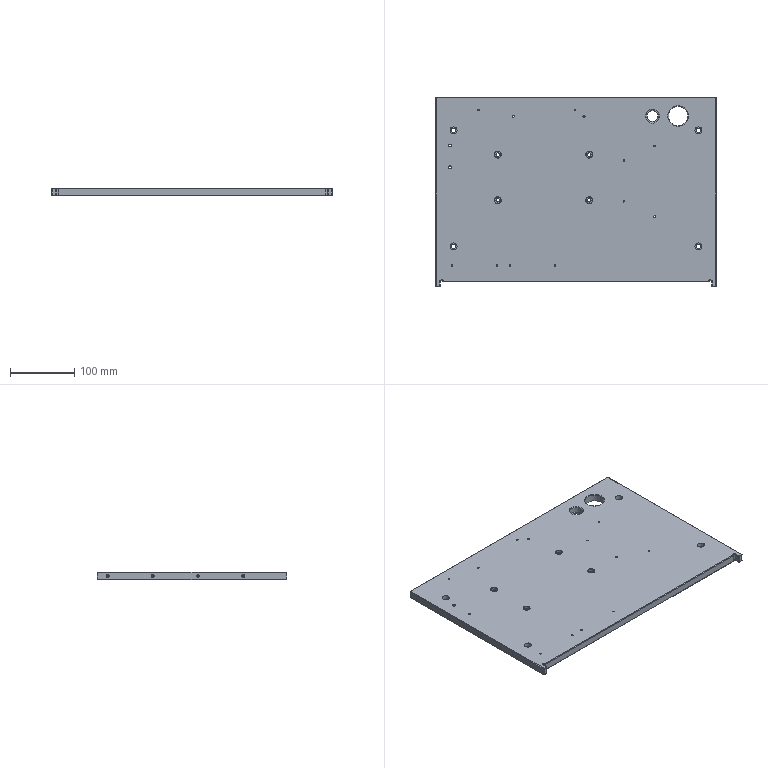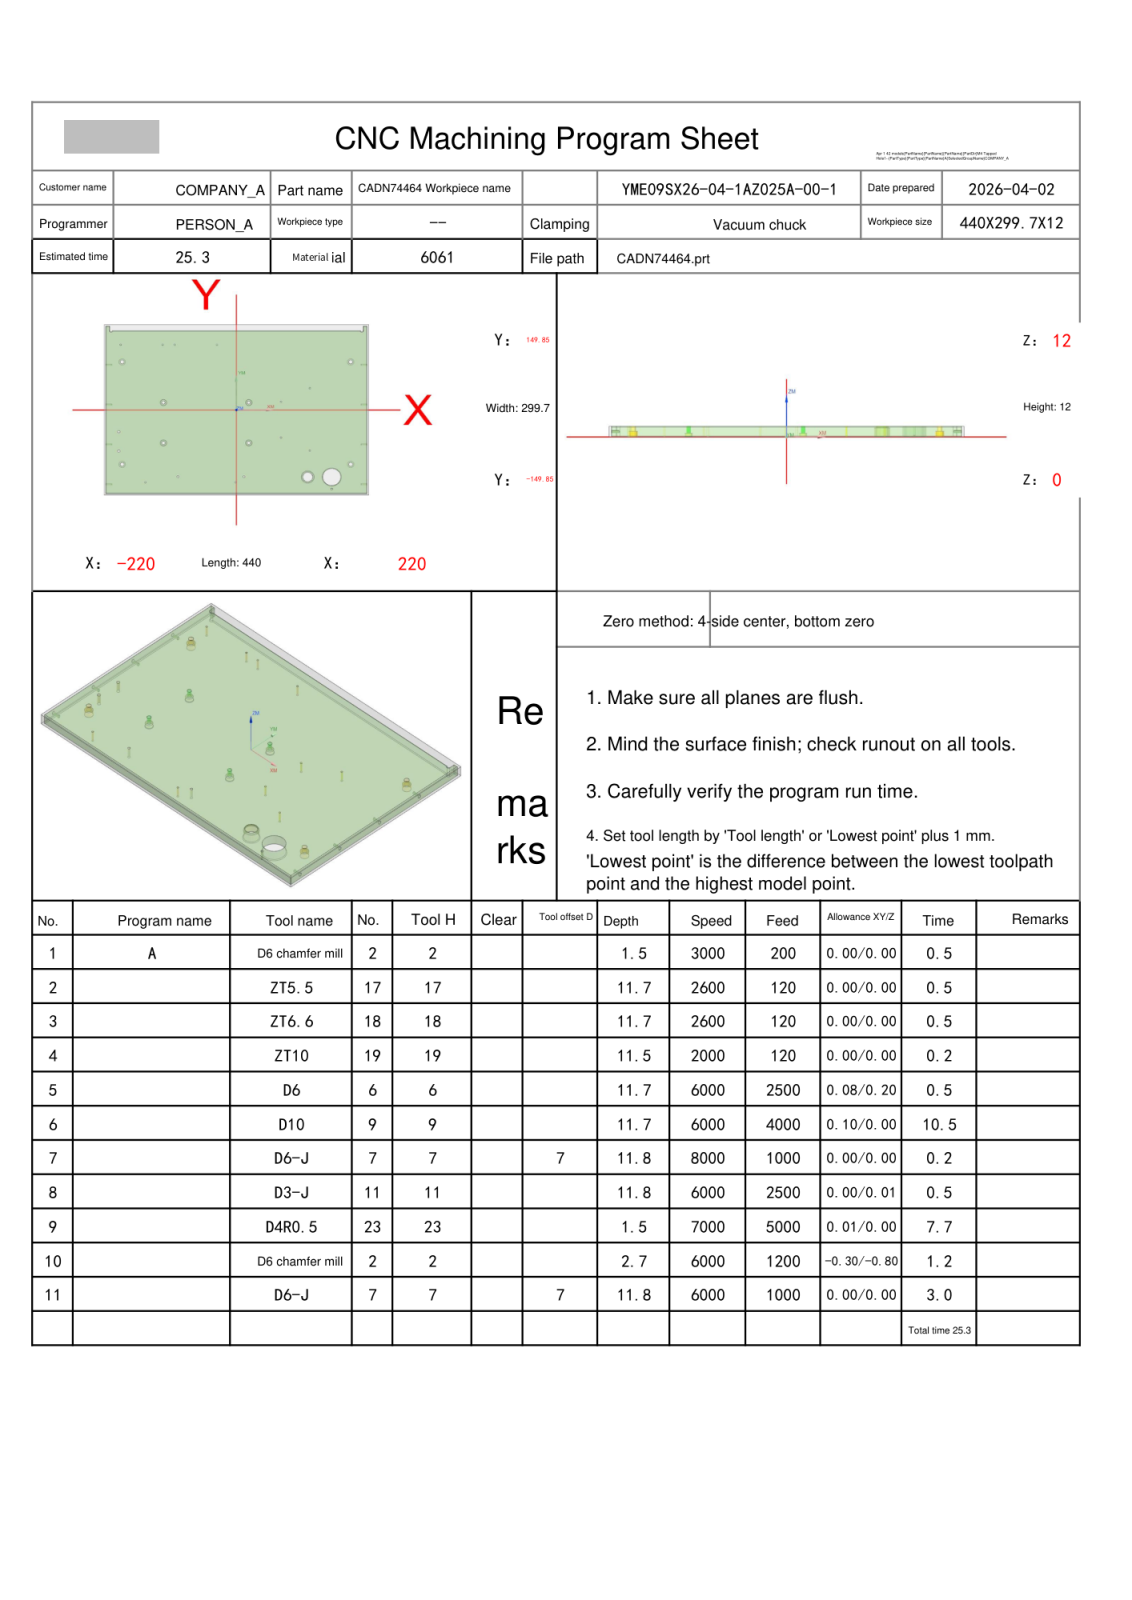NC program | NX | posted by the shop | part box 435 x 294.7 x 12 mm
Lines 896 to 1853 of 24066:
N8 T11 M06
(D3-J  D=3. R=0. H=11 ce=0.00 di=0.01)
G00 G90 G54 X-208.966 Y139.65 M03 S6000
G43 H11 Z32.
M08
Z12.471
G01 X-208.97 Y139.649 Z12.399 F2000.
X-208.981 Y139.647 Z12.326
X-208.999 Y139.642 Z12.253
X-209.022 Y139.635 Z12.182
X-209.049 Y139.626 Z12.112
X-209.078 Y139.614 Z12.046
X-209.11 Y139.599 Z11.983
X-209.142 Y139.581 Z11.924
X-209.173 Y139.559 Z11.871
X-209.203 Y139.534 Z11.824
X-209.23 Y139.506 Z11.783
X-209.253 Y139.473 Z11.75
X-209.27 Y139.437 Z11.726
X-209.282 Y139.396 Z11.71
X-209.286 Y139.35 Z11.705
G03 X-208.5 Y138.564 I.786 J0.0 F2500.
X-207.72 Y139.252 I0.0 J.786
G01 X-207.725 Y139.305 Z11.71
X-207.749 Y139.355 Z11.722
X-207.789 Y139.4 Z11.739
X-207.842 Y139.441 Z11.759
X-207.905 Y139.477 Z11.78
X-207.972 Y139.509 Z11.8
X-208.041 Y139.537 Z11.816
X-208.109 Y139.561 Z11.826
X-208.206 Y139.589 Z11.825
X-208.297 Y139.606 Z11.806
X-208.387 Y139.613 Z11.771
X-208.484 Y139.61 Z11.723
X-208.595 Y139.597 Z11.663
X-208.665 Y139.586 Z11.626
X-208.738 Y139.571 Z11.587
X-208.811 Y139.553 Z11.549
X-208.882 Y139.531 Z11.513
X-208.947 Y139.505 Z11.48
X-209.003 Y139.474 Z11.452
X-209.047 Y139.438 Z11.429
X-209.075 Y139.397 Z11.415
X-209.086 Y139.35 Z11.41
G03 X-208.5 Y138.764 I.586 J0.0
X-207.915 Y139.326 I0.0 J.586
G01 X-207.923 Y139.379 Z11.412
X-207.95 Y139.427 Z11.416
X-207.991 Y139.47 Z11.421
X-208.043 Y139.508 Z11.427
X-208.101 Y139.541 Z11.432
X-208.163 Y139.569 Z11.435
X-208.223 Y139.592
X-208.278 Y139.611 Z11.431
X-208.34 Y139.629 Z11.418
X-208.391 Y139.64 Z11.398
X-208.437 Y139.644 Z11.371
X-208.484 Y139.641 Z11.34
X-208.538 Y139.631 Z11.305
X-208.604 Y139.615 Z11.268
X-208.657 Y139.601 Z11.243
X-208.714 Y139.583 Z11.219
X-208.774 Y139.562 Z11.195
X-208.832 Y139.538 Z11.173
X-208.887 Y139.509 Z11.154
X-208.935 Y139.477 Z11.138
X-208.972 Y139.439 Z11.126
X-208.997 Y139.397 Z11.118
X-209.006 Y139.35 Z11.115
G03 X-208.5 Y138.844 I.506 J0.0
X-207.994 Y139.348 I0.0 J.506
G01 X-208.001 Y139.41 Z11.114
X-208.019 Y139.503 Z11.113
X-208.147 Y140.018 Z11.098
X-208.227 Y140.353 Z11.086
X-208.358 Y141.004 Z11.059
X-208.471 Y141.96 Z11.006
X-208.567 Y142.911 Z10.944
X-208.633 Y143.352 Z10.913
X-208.705 Y143.69 Z10.889
X-208.752 Y143.871 Z10.876
X-208.819 Y144.099 Z10.859
X-208.885 Y144.29 Z10.843
X-208.922 Y144.383 Z10.835
X-208.954 Y144.45 Z10.829
X-208.978 Y144.49 Z10.824
X-208.994 Y144.499 Z10.821
X-209. Y144.475 Z10.82
Y139.35
G03 X-208.5 Y138.85 I.5 J0.0
X-208. Y139.35 I0.0 J.5
G02 X-206.5 Y140.85 I1.5 J0.0
G01 X-205.375
X-205.346 Y140.866 Z10.819
X-205.341 Y140.911 Z10.817
X-205.358 Y140.983 Z10.812
X-205.394 Y141.078 Z10.807
X-205.449 Y141.193 Z10.8
X-205.52 Y141.325 Z10.792
X-205.702 Y141.623 Z10.774
X-205.831 Y141.816 Z10.761
X-206.055 Y142.129 Z10.74
X-206.427 Y142.585 Z10.707
X-206.833 Y143.019 Z10.673
X-207.267 Y143.425 Z10.638
X-207.722 Y143.797 Z10.605
X-208.035 Y144.021 Z10.584
X-208.228 Y144.149 Z10.571
X-208.525 Y144.331 Z10.553
X-208.657 Y144.402 Z10.545
X-208.772 Y144.456 Z10.538
X-208.867 Y144.492 Z10.533
X-208.939 Y144.509 Z10.528
X-208.984 Y144.504 Z10.526
X-209. Y144.475 Z10.525
Y139.35
G03 X-208.5 Y138.85 I.5 J0.0
X-208. Y139.35 I0.0 J.5
G02 X-206.5 Y140.85 I1.5 J0.0
G01 X-205.375
X-205.346 Y140.866 Z10.524
X-205.341 Y140.911 Z10.522
X-205.358 Y140.983 Z10.517
X-205.394 Y141.078 Z10.512
X-205.449 Y141.193 Z10.505
X-205.52 Y141.325 Z10.497
X-205.702 Y141.623 Z10.479
X-205.831 Y141.816 Z10.466
X-206.055 Y142.129 Z10.445
X-206.427 Y142.585 Z10.412
X-206.833 Y143.019 Z10.378
X-207.267 Y143.425 Z10.343
X-207.722 Y143.797 Z10.31
X-208.035 Y144.021 Z10.289
X-208.228 Y144.149 Z10.276
X-208.525 Y144.331 Z10.258
X-208.657 Y144.402 Z10.25
X-208.772 Y144.456 Z10.243
X-208.867 Y144.492 Z10.238
X-208.939 Y144.509 Z10.233
X-208.984 Y144.504 Z10.231
X-209. Y144.475 Z10.23
Y139.35
G03 X-208.5 Y138.85 I.5 J0.0
X-208. Y139.35 I0.0 J.5
G02 X-206.5 Y140.85 I1.5 J0.0
G01 X-205.375
X-205.346 Y140.866 Z10.229
X-205.341 Y140.911 Z10.227
X-205.358 Y140.983 Z10.222
X-205.394 Y141.078 Z10.217
X-205.449 Y141.193 Z10.21
X-205.52 Y141.325 Z10.202
X-205.702 Y141.623 Z10.184
X-205.831 Y141.816 Z10.171
X-206.055 Y142.129 Z10.15
X-206.427 Y142.585 Z10.117
X-206.833 Y143.019 Z10.083
X-207.267 Y143.425 Z10.048
X-207.722 Y143.797 Z10.015
X-208.035 Y144.021 Z9.994
X-208.228 Y144.149 Z9.981
X-208.525 Y144.331 Z9.963
X-208.657 Y144.402 Z9.955
X-208.772 Y144.456 Z9.948
X-208.867 Y144.492 Z9.943
X-208.939 Y144.509 Z9.938
X-208.984 Y144.504 Z9.936
X-209. Y144.475 Z9.935
Y139.35
G03 X-208.5 Y138.85 I.5 J0.0
X-208. Y139.35 I0.0 J.5
G02 X-206.5 Y140.85 I1.5 J0.0
G01 X-205.375
X-205.346 Y140.866 Z9.934
X-205.341 Y140.911 Z9.932
X-205.358 Y140.983 Z9.927
X-205.394 Y141.078 Z9.922
X-205.449 Y141.193 Z9.915
X-205.52 Y141.325 Z9.907
X-205.702 Y141.623 Z9.889
X-205.831 Y141.816 Z9.876
X-206.055 Y142.129 Z9.855
X-206.427 Y142.585 Z9.822
X-206.833 Y143.019 Z9.788
X-207.267 Y143.425 Z9.753
X-207.722 Y143.797 Z9.72
X-208.035 Y144.021 Z9.699
X-208.228 Y144.149 Z9.686
X-208.525 Y144.331 Z9.668
X-208.657 Y144.402 Z9.66
X-208.772 Y144.456 Z9.653
X-208.867 Y144.492 Z9.648
X-208.939 Y144.509 Z9.643
X-208.984 Y144.504 Z9.641
X-209. Y144.475 Z9.64
Y139.35
G03 X-208.5 Y138.85 I.5 J0.0
X-208. Y139.35 I0.0 J.5
G02 X-206.5 Y140.85 I1.5 J0.0
G01 X-205.375
X-205.346 Y140.866 Z9.639
X-205.341 Y140.911 Z9.637
X-205.358 Y140.983 Z9.632
X-205.394 Y141.078 Z9.627
X-205.449 Y141.193 Z9.62
X-205.52 Y141.325 Z9.612
X-205.702 Y141.623 Z9.594
X-205.831 Y141.816 Z9.581
X-206.055 Y142.129 Z9.56
X-206.427 Y142.585 Z9.527
X-206.833 Y143.019 Z9.493
X-207.267 Y143.425 Z9.458
X-207.722 Y143.797 Z9.425
X-208.035 Y144.021 Z9.404
X-208.228 Y144.149 Z9.391
X-208.525 Y144.331 Z9.373
X-208.657 Y144.402 Z9.365
X-208.772 Y144.456 Z9.358
X-208.867 Y144.492 Z9.353
X-208.939 Y144.509 Z9.348
X-208.984 Y144.504 Z9.346
X-209. Y144.475 Z9.345
Y139.35
G03 X-208.5 Y138.85 I.5 J0.0
X-208. Y139.35 I0.0 J.5
G02 X-206.5 Y140.85 I1.5 J0.0
G01 X-205.375
X-205.346 Y140.866 Z9.344
X-205.341 Y140.911 Z9.342
X-205.358 Y140.983 Z9.337
X-205.394 Y141.078 Z9.332
X-205.449 Y141.193 Z9.325
X-205.52 Y141.325 Z9.317
X-205.702 Y141.623 Z9.299
X-205.831 Y141.816 Z9.286
X-206.055 Y142.129 Z9.265
X-206.427 Y142.585 Z9.232
X-206.833 Y143.019 Z9.198
X-207.267 Y143.425 Z9.163
X-207.722 Y143.797 Z9.13
X-208.035 Y144.021 Z9.109
X-208.228 Y144.149 Z9.096
X-208.525 Y144.331 Z9.078
X-208.657 Y144.402 Z9.07
X-208.772 Y144.456 Z9.063
X-208.867 Y144.492 Z9.058
X-208.939 Y144.509 Z9.053
X-208.984 Y144.504 Z9.051
X-209. Y144.475 Z9.05
Y139.35
G03 X-208.5 Y138.85 I.5 J0.0
X-208. Y139.35 I0.0 J.5
G02 X-206.5 Y140.85 I1.5 J0.0
G01 X-205.375
X-205.346 Y140.866 Z9.049
X-205.341 Y140.911 Z9.047
X-205.358 Y140.983 Z9.042
X-205.394 Y141.078 Z9.037
X-205.449 Y141.193 Z9.03
X-205.52 Y141.325 Z9.022
X-205.702 Y141.623 Z9.004
X-205.831 Y141.816 Z8.991
X-206.055 Y142.129 Z8.97
X-206.427 Y142.585 Z8.937
X-206.833 Y143.019 Z8.903
X-207.267 Y143.425 Z8.868
X-207.722 Y143.797 Z8.835
X-208.035 Y144.021 Z8.814
X-208.228 Y144.149 Z8.801
X-208.525 Y144.331 Z8.783
X-208.657 Y144.402 Z8.775
X-208.772 Y144.456 Z8.768
X-208.867 Y144.492 Z8.763
X-208.939 Y144.509 Z8.758
X-208.984 Y144.504 Z8.756
X-209. Y144.475 Z8.755
Y139.35
G03 X-208.5 Y138.85 I.5 J0.0
X-208. Y139.35 I0.0 J.5
G02 X-206.5 Y140.85 I1.5 J0.0
G01 X-205.375
X-205.346 Y140.866 Z8.754
X-205.341 Y140.911 Z8.752
X-205.358 Y140.983 Z8.747
X-205.394 Y141.078 Z8.742
X-205.449 Y141.193 Z8.735
X-205.52 Y141.325 Z8.727
X-205.702 Y141.623 Z8.709
X-205.831 Y141.816 Z8.696
X-206.055 Y142.129 Z8.675
X-206.427 Y142.585 Z8.642
X-206.833 Y143.019 Z8.608
X-207.267 Y143.425 Z8.573
X-207.722 Y143.797 Z8.54
X-208.035 Y144.021 Z8.519
X-208.228 Y144.149 Z8.506
X-208.525 Y144.331 Z8.488
X-208.657 Y144.402 Z8.48
X-208.772 Y144.456 Z8.473
X-208.867 Y144.492 Z8.468
X-208.939 Y144.509 Z8.463
X-208.984 Y144.504 Z8.461
X-209. Y144.475 Z8.46
Y139.35
G03 X-208.5 Y138.85 I.5 J0.0
X-208. Y139.35 I0.0 J.5
G02 X-206.5 Y140.85 I1.5 J0.0
G01 X-205.375
X-205.346 Y140.866 Z8.459
X-205.341 Y140.911 Z8.457
X-205.358 Y140.983 Z8.452
X-205.394 Y141.078 Z8.447
X-205.449 Y141.193 Z8.44
X-205.52 Y141.325 Z8.432
X-205.702 Y141.623 Z8.414
X-205.831 Y141.816 Z8.401
X-206.055 Y142.129 Z8.38
X-206.427 Y142.585 Z8.347
X-206.833 Y143.019 Z8.313
X-207.267 Y143.425 Z8.278
X-207.722 Y143.797 Z8.245
X-208.035 Y144.021 Z8.224
X-208.228 Y144.149 Z8.211
X-208.525 Y144.331 Z8.193
X-208.657 Y144.402 Z8.185
X-208.772 Y144.456 Z8.178
X-208.867 Y144.492 Z8.173
X-208.939 Y144.509 Z8.168
X-208.984 Y144.504 Z8.166
X-209. Y144.475 Z8.165
Y139.35
G03 X-208.5 Y138.85 I.5 J0.0
X-208. Y139.35 I0.0 J.5
G02 X-206.5 Y140.85 I1.5 J0.0
G01 X-205.375
X-205.346 Y140.866 Z8.164
X-205.341 Y140.911 Z8.162
X-205.358 Y140.983 Z8.157
X-205.394 Y141.078 Z8.152
X-205.449 Y141.193 Z8.145
X-205.52 Y141.325 Z8.137
X-205.702 Y141.623 Z8.119
X-205.831 Y141.816 Z8.106
X-206.055 Y142.129 Z8.085
X-206.427 Y142.585 Z8.052
X-206.833 Y143.019 Z8.018
X-207.267 Y143.425 Z7.983
X-207.722 Y143.797 Z7.95
X-208.035 Y144.021 Z7.929
X-208.228 Y144.149 Z7.916
X-208.525 Y144.331 Z7.898
X-208.657 Y144.402 Z7.89
X-208.772 Y144.456 Z7.883
X-208.867 Y144.492 Z7.878
X-208.939 Y144.509 Z7.873
X-208.984 Y144.504 Z7.871
X-209. Y144.475 Z7.87
Y139.35
G03 X-208.5 Y138.85 I.5 J0.0
X-208. Y139.35 I0.0 J.5
G02 X-206.5 Y140.85 I1.5 J0.0
G01 X-205.375
X-205.346 Y140.866 Z7.869
X-205.341 Y140.911 Z7.867
X-205.358 Y140.983 Z7.862
X-205.394 Y141.078 Z7.857
X-205.449 Y141.193 Z7.85
X-205.52 Y141.325 Z7.842
X-205.702 Y141.623 Z7.824
X-205.831 Y141.816 Z7.811
X-206.055 Y142.129 Z7.79
X-206.427 Y142.585 Z7.757
X-206.833 Y143.019 Z7.723
X-207.267 Y143.425 Z7.688
X-207.722 Y143.797 Z7.655
X-208.035 Y144.021 Z7.634
X-208.228 Y144.149 Z7.621
X-208.525 Y144.331 Z7.603
X-208.657 Y144.402 Z7.595
X-208.772 Y144.456 Z7.588
X-208.867 Y144.492 Z7.583
X-208.939 Y144.509 Z7.578
X-208.984 Y144.504 Z7.576
X-209. Y144.475 Z7.575
Y139.35
G03 X-208.5 Y138.85 I.5 J0.0
X-208. Y139.35 I0.0 J.5
G02 X-206.5 Y140.85 I1.5 J0.0
G01 X-205.375
X-205.346 Y140.866 Z7.574
X-205.341 Y140.911 Z7.572
X-205.358 Y140.983 Z7.567
X-205.394 Y141.078 Z7.562
X-205.449 Y141.193 Z7.555
X-205.52 Y141.325 Z7.547
X-205.702 Y141.623 Z7.529
X-205.831 Y141.816 Z7.516
X-206.055 Y142.129 Z7.495
X-206.427 Y142.585 Z7.462
X-206.833 Y143.019 Z7.428
X-207.267 Y143.425 Z7.393
X-207.722 Y143.797 Z7.36
X-208.035 Y144.021 Z7.339
X-208.228 Y144.149 Z7.326
X-208.525 Y144.331 Z7.308
X-208.657 Y144.402 Z7.3
X-208.772 Y144.456 Z7.293
X-208.867 Y144.492 Z7.288
X-208.939 Y144.509 Z7.283
X-208.984 Y144.504 Z7.281
X-209. Y144.475 Z7.28
Y139.35
G03 X-208.5 Y138.85 I.5 J0.0
X-208. Y139.35 I0.0 J.5
G02 X-206.5 Y140.85 I1.5 J0.0
G01 X-205.375
X-205.346 Y140.866 Z7.279
X-205.341 Y140.911 Z7.277
X-205.358 Y140.983 Z7.272
X-205.394 Y141.078 Z7.267
X-205.449 Y141.193 Z7.26
X-205.52 Y141.325 Z7.252
X-205.702 Y141.623 Z7.234
X-205.831 Y141.816 Z7.221
X-206.055 Y142.129 Z7.2
X-206.427 Y142.585 Z7.167
X-206.833 Y143.019 Z7.133
X-207.267 Y143.425 Z7.098
X-207.722 Y143.797 Z7.065
X-208.035 Y144.021 Z7.044
X-208.228 Y144.149 Z7.031
X-208.525 Y144.331 Z7.013
X-208.657 Y144.402 Z7.005
X-208.772 Y144.456 Z6.998
X-208.867 Y144.492 Z6.993
X-208.939 Y144.509 Z6.988
X-208.984 Y144.504 Z6.986
X-209. Y144.475 Z6.985
Y139.35
G03 X-208.5 Y138.85 I.5 J0.0
X-208. Y139.35 I0.0 J.5
G02 X-206.5 Y140.85 I1.5 J0.0
G01 X-205.375
X-205.346 Y140.866 Z6.984
X-205.341 Y140.911 Z6.982
X-205.358 Y140.983 Z6.977
X-205.394 Y141.078 Z6.972
X-205.449 Y141.193 Z6.965
X-205.52 Y141.325 Z6.957
X-205.702 Y141.623 Z6.939
X-205.831 Y141.816 Z6.926
X-206.055 Y142.129 Z6.905
X-206.427 Y142.585 Z6.872
X-206.833 Y143.019 Z6.838
X-207.267 Y143.425 Z6.803
X-207.722 Y143.797 Z6.77
X-208.035 Y144.021 Z6.749
X-208.228 Y144.149 Z6.736
X-208.525 Y144.331 Z6.718
X-208.657 Y144.402 Z6.71
X-208.772 Y144.456 Z6.703
X-208.867 Y144.492 Z6.698
X-208.939 Y144.509 Z6.693
X-208.984 Y144.504 Z6.691
X-209. Y144.475 Z6.69
Y139.35
G03 X-208.5 Y138.85 I.5 J0.0
X-208. Y139.35 I0.0 J.5
G02 X-206.5 Y140.85 I1.5 J0.0
G01 X-205.375
X-205.346 Y140.866 Z6.689
X-205.341 Y140.911 Z6.687
X-205.358 Y140.983 Z6.682
X-205.394 Y141.078 Z6.677
X-205.449 Y141.193 Z6.67
X-205.52 Y141.325 Z6.662
X-205.702 Y141.623 Z6.644
X-205.831 Y141.816 Z6.631
X-206.055 Y142.129 Z6.61
X-206.427 Y142.585 Z6.577
X-206.833 Y143.019 Z6.543
X-207.267 Y143.425 Z6.508
X-207.722 Y143.797 Z6.475
X-208.035 Y144.021 Z6.454
X-208.228 Y144.149 Z6.441
X-208.525 Y144.331 Z6.423
X-208.657 Y144.402 Z6.415
X-208.772 Y144.456 Z6.408
X-208.867 Y144.492 Z6.403
X-208.939 Y144.509 Z6.398
X-208.984 Y144.504 Z6.396
X-209. Y144.475 Z6.395
Y139.35
G03 X-208.5 Y138.85 I.5 J0.0
X-208. Y139.35 I0.0 J.5
G02 X-206.5 Y140.85 I1.5 J0.0
G01 X-205.375
X-205.346 Y140.866 Z6.394
X-205.341 Y140.911 Z6.392
X-205.358 Y140.983 Z6.387
X-205.394 Y141.078 Z6.382
X-205.449 Y141.193 Z6.375
X-205.52 Y141.325 Z6.367
X-205.702 Y141.623 Z6.349
X-205.831 Y141.816 Z6.336
X-206.055 Y142.129 Z6.315
X-206.427 Y142.585 Z6.282
X-206.833 Y143.019 Z6.248
X-207.267 Y143.425 Z6.213
X-207.722 Y143.797 Z6.18
X-208.035 Y144.021 Z6.159
X-208.228 Y144.149 Z6.146
X-208.525 Y144.331 Z6.128
X-208.657 Y144.402 Z6.12
X-208.772 Y144.456 Z6.113
X-208.867 Y144.492 Z6.108
X-208.939 Y144.509 Z6.103
X-208.984 Y144.504 Z6.101
X-209. Y144.475 Z6.1
Y139.35
G03 X-208.5 Y138.85 I.5 J0.0
X-208. Y139.35 I0.0 J.5
G02 X-206.5 Y140.85 I1.5 J0.0
G01 X-205.375
X-205.346 Y140.866 Z6.099
X-205.341 Y140.911 Z6.097
X-205.358 Y140.983 Z6.092
X-205.394 Y141.078 Z6.087
X-205.449 Y141.193 Z6.08
X-205.52 Y141.325 Z6.072
X-205.702 Y141.623 Z6.054
X-205.831 Y141.816 Z6.041
X-206.055 Y142.129 Z6.02
X-206.427 Y142.585 Z5.987
X-206.833 Y143.019 Z5.953
X-207.267 Y143.425 Z5.918
X-207.722 Y143.797 Z5.885
X-208.035 Y144.021 Z5.864
X-208.228 Y144.149 Z5.851
X-208.525 Y144.331 Z5.833
X-208.657 Y144.402 Z5.825
X-208.772 Y144.456 Z5.818
X-208.867 Y144.492 Z5.813
X-208.939 Y144.509 Z5.808
X-208.984 Y144.504 Z5.806
X-209. Y144.475 Z5.805
Y139.35
G03 X-208.5 Y138.85 I.5 J0.0
X-208. Y139.35 I0.0 J.5
G02 X-206.5 Y140.85 I1.5 J0.0
G01 X-205.375
X-205.346 Y140.866 Z5.804
X-205.341 Y140.911 Z5.802
X-205.358 Y140.983 Z5.797
X-205.394 Y141.078 Z5.792
X-205.449 Y141.193 Z5.785
X-205.52 Y141.325 Z5.777
X-205.702 Y141.623 Z5.759
X-205.831 Y141.816 Z5.746
X-206.055 Y142.129 Z5.725
X-206.427 Y142.585 Z5.692
X-206.833 Y143.019 Z5.658
X-207.267 Y143.425 Z5.623
X-207.722 Y143.797 Z5.59
X-208.035 Y144.021 Z5.569
X-208.228 Y144.149 Z5.556
X-208.525 Y144.331 Z5.538
X-208.657 Y144.402 Z5.53
X-208.772 Y144.456 Z5.523
X-208.867 Y144.492 Z5.518
X-208.939 Y144.509 Z5.513
X-208.984 Y144.504 Z5.511
X-209. Y144.475 Z5.51
Y139.35
G03 X-208.5 Y138.85 I.5 J0.0
X-208. Y139.35 I0.0 J.5
G02 X-206.5 Y140.85 I1.5 J0.0
G01 X-205.375
X-205.346 Y140.866 Z5.509
X-205.341 Y140.911 Z5.507
X-205.358 Y140.983 Z5.502
X-205.394 Y141.078 Z5.497
X-205.449 Y141.193 Z5.49
X-205.52 Y141.325 Z5.482
X-205.702 Y141.623 Z5.464
X-205.831 Y141.816 Z5.451
X-206.055 Y142.129 Z5.43
X-206.427 Y142.585 Z5.397
X-206.833 Y143.019 Z5.363
X-207.267 Y143.425 Z5.328
X-207.722 Y143.797 Z5.295
X-208.035 Y144.021 Z5.274
X-208.228 Y144.149 Z5.261
X-208.525 Y144.331 Z5.243
X-208.657 Y144.402 Z5.235
X-208.772 Y144.456 Z5.228
X-208.867 Y144.492 Z5.223
X-208.939 Y144.509 Z5.218
X-208.984 Y144.504 Z5.216
X-209. Y144.475 Z5.215
Y139.35
G03 X-208.5 Y138.85 I.5 J0.0
X-208. Y139.35 I0.0 J.5
G02 X-206.5 Y140.85 I1.5 J0.0
G01 X-205.375
X-205.346 Y140.866 Z5.214
X-205.341 Y140.911 Z5.212
X-205.358 Y140.983 Z5.207
X-205.394 Y141.078 Z5.202
X-205.449 Y141.193 Z5.195
X-205.52 Y141.325 Z5.187
X-205.702 Y141.623 Z5.169
X-205.831 Y141.816 Z5.156
X-206.055 Y142.129 Z5.135
X-206.427 Y142.585 Z5.102
X-206.833 Y143.019 Z5.068
X-207.267 Y143.425 Z5.033
X-207.722 Y143.797 Z5.
X-208.035 Y144.021 Z4.979
X-208.228 Y144.149 Z4.966
X-208.525 Y144.331 Z4.948
X-208.657 Y144.402 Z4.94
X-208.772 Y144.456 Z4.933
X-208.867 Y144.492 Z4.928
X-208.939 Y144.509 Z4.923
X-208.984 Y144.504 Z4.921
X-209. Y144.475 Z4.92
Y139.35
G03 X-208.5 Y138.85 I.5 J0.0
X-208. Y139.35 I0.0 J.5
G02 X-206.5 Y140.85 I1.5 J0.0
G01 X-205.375
X-205.346 Y140.866 Z4.919
X-205.341 Y140.911 Z4.917
X-205.358 Y140.983 Z4.912
X-205.394 Y141.078 Z4.907
X-205.449 Y141.193 Z4.9
X-205.52 Y141.325 Z4.892
X-205.702 Y141.623 Z4.874
X-205.831 Y141.816 Z4.861
X-206.055 Y142.129 Z4.84
X-206.427 Y142.585 Z4.807
X-206.833 Y143.019 Z4.773
X-207.267 Y143.425 Z4.738
X-207.722 Y143.797 Z4.705
X-208.035 Y144.021 Z4.684
X-208.228 Y144.149 Z4.671
X-208.525 Y144.331 Z4.653
X-208.657 Y144.402 Z4.645
X-208.772 Y144.456 Z4.638
X-208.867 Y144.492 Z4.633
X-208.939 Y144.509 Z4.628
X-208.984 Y144.504 Z4.626
X-209. Y144.475 Z4.625
Y139.35
G03 X-208.5 Y138.85 I.5 J0.0
X-208. Y139.35 I0.0 J.5
G02 X-206.5 Y140.85 I1.5 J0.0
G01 X-205.375
X-205.346 Y140.866 Z4.624
X-205.341 Y140.911 Z4.622
X-205.358 Y140.983 Z4.617
X-205.394 Y141.078 Z4.612
X-205.449 Y141.193 Z4.605
X-205.52 Y141.325 Z4.597
X-205.702 Y141.623 Z4.579
X-205.831 Y141.816 Z4.566
X-206.055 Y142.129 Z4.545
X-206.427 Y142.585 Z4.512
X-206.833 Y143.019 Z4.478
X-207.267 Y143.425 Z4.443
X-207.722 Y143.797 Z4.41
X-208.035 Y144.021 Z4.389
X-208.228 Y144.149 Z4.376
X-208.525 Y144.331 Z4.358
X-208.657 Y144.402 Z4.35
X-208.772 Y144.456 Z4.343
X-208.867 Y144.492 Z4.338
X-208.939 Y144.509 Z4.333
X-208.984 Y144.504 Z4.331
X-209. Y144.475 Z4.33
Y139.35
G03 X-208.5 Y138.85 I.5 J0.0
X-208. Y139.35 I0.0 J.5
G02 X-206.5 Y140.85 I1.5 J0.0
G01 X-205.375
X-205.346 Y140.866 Z4.329
X-205.341 Y140.911 Z4.327
X-205.358 Y140.983 Z4.322
X-205.394 Y141.078 Z4.317
X-205.449 Y141.193 Z4.31
X-205.52 Y141.325 Z4.302
X-205.702 Y141.623 Z4.284
X-205.831 Y141.816 Z4.271
X-206.055 Y142.129 Z4.25
X-206.427 Y142.585 Z4.217
X-206.833 Y143.019 Z4.183
X-207.267 Y143.425 Z4.148
X-207.722 Y143.797 Z4.115
X-208.035 Y144.021 Z4.094
X-208.228 Y144.149 Z4.081
X-208.525 Y144.331 Z4.063
X-208.657 Y144.402 Z4.055
X-208.772 Y144.456 Z4.048
X-208.867 Y144.492 Z4.043
X-208.939 Y144.509 Z4.038
X-208.984 Y144.504 Z4.036
X-209. Y144.475 Z4.035
Y139.35
G03 X-208.5 Y138.85 I.5 J0.0
X-208. Y139.35 I0.0 J.5
G02 X-206.5 Y140.85 I1.5 J0.0
G01 X-205.375
X-205.346 Y140.866 Z4.034
X-205.341 Y140.911 Z4.032
X-205.358 Y140.983 Z4.027
X-205.394 Y141.078 Z4.022
X-205.449 Y141.193 Z4.015
X-205.52 Y141.325 Z4.007
X-205.702 Y141.623 Z3.989
X-205.831 Y141.816 Z3.976
X-206.055 Y142.129 Z3.955
X-206.427 Y142.585 Z3.922
X-206.833 Y143.019 Z3.888
X-207.267 Y143.425 Z3.853
X-207.722 Y143.797 Z3.82
X-208.035 Y144.021 Z3.799
X-208.228 Y144.149 Z3.786
X-208.525 Y144.331 Z3.768
X-208.657 Y144.402 Z3.76
X-208.772 Y144.456 Z3.753
X-208.867 Y144.492 Z3.748
X-208.939 Y144.509 Z3.743
X-208.984 Y144.504 Z3.741
X-209. Y144.475 Z3.74
Y139.35
G03 X-208.5 Y138.85 I.5 J0.0
X-208. Y139.35 I0.0 J.5
G02 X-206.5 Y140.85 I1.5 J0.0
G01 X-205.375
X-205.346 Y140.866 Z3.739
X-205.341 Y140.911 Z3.737
X-205.358 Y140.983 Z3.732
X-205.394 Y141.078 Z3.727
X-205.449 Y141.193 Z3.72
X-205.52 Y141.325 Z3.712
X-205.702 Y141.623 Z3.694
X-205.831 Y141.816 Z3.681
X-206.055 Y142.129 Z3.66
X-206.427 Y142.585 Z3.627
X-206.833 Y143.019 Z3.593
X-207.267 Y143.425 Z3.558
X-207.722 Y143.797 Z3.525
X-208.035 Y144.021 Z3.504
X-208.228 Y144.149 Z3.491
X-208.525 Y144.331 Z3.473
X-208.657 Y144.402 Z3.465
X-208.772 Y144.456 Z3.458
X-208.867 Y144.492 Z3.453
X-208.939 Y144.509 Z3.448
X-208.984 Y144.504 Z3.446
X-209. Y144.475 Z3.445
Y139.35
G03 X-208.5 Y138.85 I.5 J0.0
X-208. Y139.35 I0.0 J.5
G02 X-206.5 Y140.85 I1.5 J0.0
G01 X-205.375
X-205.346 Y140.866 Z3.444
X-205.341 Y140.911 Z3.442
X-205.358 Y140.983 Z3.437
X-205.394 Y141.078 Z3.432
X-205.449 Y141.193 Z3.425
X-205.52 Y141.325 Z3.417
X-205.702 Y141.623 Z3.399
X-205.831 Y141.816 Z3.386
X-206.055 Y142.129 Z3.365
X-206.427 Y142.585 Z3.332
X-206.833 Y143.019 Z3.298
X-207.267 Y143.425 Z3.263
X-207.722 Y143.797 Z3.23
X-208.035 Y144.021 Z3.209
X-208.228 Y144.149 Z3.196
X-208.525 Y144.331 Z3.178
X-208.657 Y144.402 Z3.17
X-208.772 Y144.456 Z3.163
X-208.867 Y144.492 Z3.158
X-208.939 Y144.509 Z3.153
X-208.984 Y144.504 Z3.151
X-209. Y144.475 Z3.15
Y139.35
G03 X-208.5 Y138.85 I.5 J0.0
X-208. Y139.35 I0.0 J.5
G02 X-206.5 Y140.85 I1.5 J0.0
G01 X-205.375
X-205.346 Y140.866 Z3.149
X-205.341 Y140.911 Z3.147
X-205.358 Y140.983 Z3.142
X-205.394 Y141.078 Z3.137
X-205.449 Y141.193 Z3.13
X-205.52 Y141.325 Z3.122
X-205.702 Y141.623 Z3.104
X-205.831 Y141.816 Z3.091
X-206.055 Y142.129 Z3.07
X-206.427 Y142.585 Z3.037
X-206.833 Y143.019 Z3.003
X-207.267 Y143.425 Z2.968
X-207.722 Y143.797 Z2.935
X-208.035 Y144.021 Z2.914
X-208.228 Y144.149 Z2.901
X-208.525 Y144.331 Z2.883
X-208.657 Y144.402 Z2.875
X-208.772 Y144.456 Z2.868
X-208.867 Y144.492 Z2.863
X-208.939 Y144.509 Z2.858
X-208.984 Y144.504 Z2.856
X-209. Y144.475 Z2.855
Y139.35
G03 X-208.5 Y138.85 I.5 J0.0
X-208. Y139.35 I0.0 J.5
G02 X-206.5 Y140.85 I1.5 J0.0
G01 X-205.375
X-205.346 Y140.866 Z2.854
X-205.341 Y140.911 Z2.852
X-205.358 Y140.983 Z2.847
X-205.394 Y141.078 Z2.842
X-205.449 Y141.193 Z2.835
X-205.52 Y141.325 Z2.827
X-205.702 Y141.623 Z2.809
X-205.831 Y141.816 Z2.796
X-206.055 Y142.129 Z2.775
X-206.427 Y142.585 Z2.742
X-206.833 Y143.019 Z2.708
X-207.267 Y143.425 Z2.673
X-207.722 Y143.797 Z2.64
X-208.035 Y144.021 Z2.619
X-208.228 Y144.149 Z2.606
X-208.525 Y144.331 Z2.588
X-208.657 Y144.402 Z2.58
X-208.772 Y144.456 Z2.573
X-208.867 Y144.492 Z2.568
X-208.939 Y144.509 Z2.563
X-208.984 Y144.504 Z2.561
X-209. Y144.475 Z2.56
Y139.35
G03 X-208.5 Y138.85 I.5 J0.0
X-208. Y139.35 I0.0 J.5
G02 X-206.5 Y140.85 I1.5 J0.0
G01 X-205.375
X-205.346 Y140.866 Z2.559
X-205.341 Y140.911 Z2.557
X-205.358 Y140.983 Z2.552
X-205.394 Y141.078 Z2.547
X-205.449 Y141.193 Z2.54
X-205.52 Y141.325 Z2.532
X-205.702 Y141.623 Z2.514
X-205.831 Y141.816 Z2.501
X-206.055 Y142.129 Z2.48
X-206.427 Y142.585 Z2.447
X-206.833 Y143.019 Z2.413
X-207.267 Y143.425 Z2.378
X-207.722 Y143.797 Z2.345
X-208.035 Y144.021 Z2.324
X-208.228 Y144.149 Z2.311
X-208.525 Y144.331 Z2.293
X-208.657 Y144.402 Z2.285
X-208.772 Y144.456 Z2.278
X-208.867 Y144.492 Z2.273
X-208.939 Y144.509 Z2.268
X-208.984 Y144.504 Z2.266
X-209. Y144.475 Z2.265
Y139.35
G03 X-208.5 Y138.85 I.5 J0.0
X-208. Y139.35 I0.0 J.5
G02 X-206.5 Y140.85 I1.5 J0.0
G01 X-205.375
X-205.346 Y140.866 Z2.264
X-205.341 Y140.911 Z2.262
X-205.358 Y140.983 Z2.257
X-205.394 Y141.078 Z2.252
X-205.449 Y141.193 Z2.245
X-205.52 Y141.325 Z2.237
X-205.702 Y141.623 Z2.219
X-205.831 Y141.816 Z2.206
X-206.055 Y142.129 Z2.185
X-206.427 Y142.585 Z2.152
X-206.833 Y143.019 Z2.118
X-207.267 Y143.425 Z2.083
X-207.722 Y143.797 Z2.05
X-208.035 Y144.021 Z2.029
X-208.228 Y144.149 Z2.016
X-208.525 Y144.331 Z1.998
X-208.657 Y144.402 Z1.99
X-208.772 Y144.456 Z1.983
X-208.867 Y144.492 Z1.978
X-208.939 Y144.509 Z1.973
X-208.984 Y144.504 Z1.971
X-209. Y144.475 Z1.97
Y139.35
G03 X-208.5 Y138.85 I.5 J0.0
X-208. Y139.35 I0.0 J.5
G02 X-206.5 Y140.85 I1.5 J0.0
G01 X-205.375
X-205.346 Y140.866 Z1.969
X-205.341 Y140.911 Z1.967
X-205.358 Y140.983 Z1.962
X-205.394 Y141.078 Z1.957
X-205.449 Y141.193 Z1.95
X-205.52 Y141.325 Z1.942
X-205.702 Y141.623 Z1.924
X-205.831 Y141.816 Z1.911
X-206.055 Y142.129 Z1.89
X-206.427 Y142.585 Z1.857
X-206.833 Y143.019 Z1.823
X-207.267 Y143.425 Z1.788
X-207.722 Y143.797 Z1.755
X-208.035 Y144.021 Z1.734
X-208.228 Y144.149 Z1.721
X-208.525 Y144.331 Z1.703
X-208.657 Y144.402 Z1.695
X-208.772 Y144.456 Z1.688
X-208.867 Y144.492 Z1.683
X-208.939 Y144.509 Z1.678
X-208.984 Y144.504 Z1.676
X-209. Y144.475 Z1.675
Y139.35
G03 X-208.5 Y138.85 I.5 J0.0
X-208. Y139.35 I0.0 J.5
G02 X-206.5 Y140.85 I1.5 J0.0
G01 X-205.375
X-205.346 Y140.866 Z1.674
X-205.341 Y140.911 Z1.672
X-205.358 Y140.983 Z1.667
X-205.394 Y141.078 Z1.662
X-205.449 Y141.193 Z1.655
X-205.52 Y141.325 Z1.647
X-205.702 Y141.623 Z1.629
X-205.831 Y141.816 Z1.616
X-206.055 Y142.129 Z1.595
X-206.427 Y142.585 Z1.562
X-206.833 Y143.019 Z1.528
X-207.267 Y143.425 Z1.493
X-207.722 Y143.797 Z1.46
X-208.035 Y144.021 Z1.439
X-208.228 Y144.149 Z1.426
X-208.525 Y144.331 Z1.408
X-208.657 Y144.402 Z1.4
X-208.772 Y144.456 Z1.393
X-208.867 Y144.492 Z1.388
X-208.939 Y144.509 Z1.383
X-208.984 Y144.504 Z1.381
X-209. Y144.475 Z1.38
Y139.35
G03 X-208.5 Y138.85 I.5 J0.0
X-208. Y139.35 I0.0 J.5
G02 X-206.5 Y140.85 I1.5 J0.0
G01 X-205.375